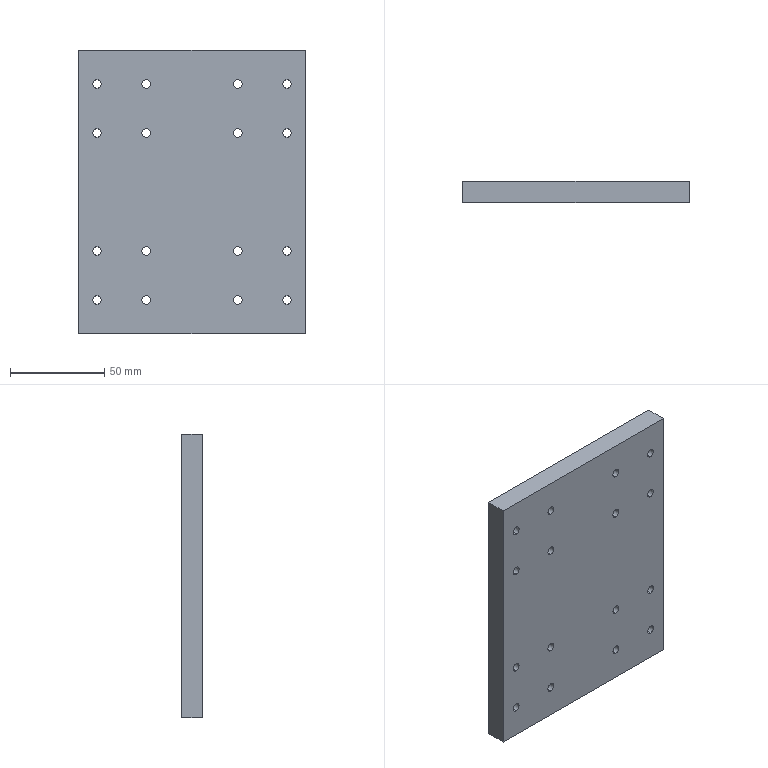Part | STEP file | csb-00003 | 1 solid | 86 faces | box 120 x 11 x 150 mm | volume 192672 mm3 | cylinder 64 | plane 22 | commonest cylinder face diameters 4.5 x32 8 x32